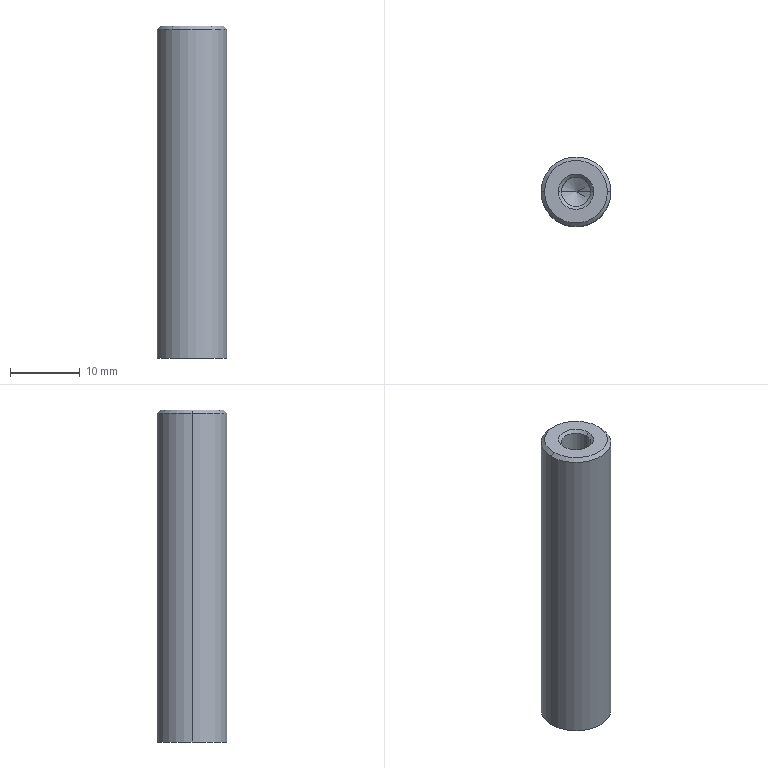Part | 1 solid | 12 faces | box 10 x 10 x 47.5 mm | volume 3479 mm3 | cone 6 | cylinder 4 | plane 2 | commonest cylinder face diameters 4.2 x2 10 x2
STEP:
#1=CARTESIAN_POINT('',(-2.1,0.,47.075));
#2=VERTEX_POINT('',#1);
#3=CARTESIAN_POINT('',(2.1,0.,47.075));
#4=VERTEX_POINT('',#3);
#5=CARTESIAN_POINT('',(0.,0.,47.075));
#6=DIRECTION('',(0.,0.,1.));
#7=DIRECTION('',(1.,0.,0.));
#8=AXIS2_PLACEMENT_3D('',#5,#6,#7);
#9=CIRCLE('',#8,2.1);
#10=EDGE_CURVE('',#2,#4,#9,.T.);
#11=ORIENTED_EDGE('',*,*,#10,.F.);
#12=CARTESIAN_POINT('',(-2.525,0.,47.5));
#13=VERTEX_POINT('',#12);
#14=CARTESIAN_POINT('',(-2.525,0.,47.5));
#15=DIRECTION('',(-0.7071,0.,0.7071));
#16=VECTOR('',#15,1000.);
#17=LINE('',#14,#16);
#18=EDGE_CURVE('',#2,#13,#17,.T.);
#19=ORIENTED_EDGE('',*,*,#18,.T.);
#20=CARTESIAN_POINT('',(2.525,0.,47.5));
#21=VERTEX_POINT('',#20);
#22=CARTESIAN_POINT('',(0.,0.,47.5));
#23=DIRECTION('',(0.,0.,1.));
#24=DIRECTION('',(1.,0.,0.));
#25=AXIS2_PLACEMENT_3D('',#22,#23,#24);
#26=CIRCLE('',#25,2.525);
#27=EDGE_CURVE('',#13,#21,#26,.T.);
#28=ORIENTED_EDGE('',*,*,#27,.T.);
#29=CARTESIAN_POINT('',(2.525,0.,47.5));
#30=DIRECTION('',(0.7071,0.,0.7071));
#31=VECTOR('',#30,1000.);
#32=LINE('',#29,#31);
#33=EDGE_CURVE('',#4,#21,#32,.T.);
#34=ORIENTED_EDGE('',*,*,#33,.F.);
#35=EDGE_LOOP('',(#11,#19,#28,#34));
#36=FACE_OUTER_BOUND('',#35,.T.);
#37=CARTESIAN_POINT('',(0.,0.,47.5));
#38=DIRECTION('',(0.,0.,1.));
#39=DIRECTION('',(1.,0.,0.));
#40=AXIS2_PLACEMENT_3D('',#37,#38,#39);
#41=CONICAL_SURFACE('',#40,2.525,0.7854);
#42=ADVANCED_FACE('',(#36),#41,.F.);
#43=CARTESIAN_POINT('',(-2.1,0.,30.1));
#44=VERTEX_POINT('',#43);
#45=CARTESIAN_POINT('',(2.1,0.,30.1));
#46=VERTEX_POINT('',#45);
#47=CARTESIAN_POINT('',(0.,0.,30.1));
#48=DIRECTION('',(0.,0.,1.));
#49=DIRECTION('',(1.,0.,0.));
#50=AXIS2_PLACEMENT_3D('',#47,#48,#49);
#51=CIRCLE('',#50,2.1);
#52=EDGE_CURVE('',#44,#46,#51,.T.);
#53=ORIENTED_EDGE('',*,*,#52,.F.);
#54=CARTESIAN_POINT('',(-2.1,0.,47.5));
#55=DIRECTION('',(0.,0.,1.));
#56=VECTOR('',#55,1000.);
#57=LINE('',#54,#56);
#58=EDGE_CURVE('',#44,#2,#57,.T.);
#59=ORIENTED_EDGE('',*,*,#58,.T.);
#60=ORIENTED_EDGE('',*,*,#10,.T.);
#61=CARTESIAN_POINT('',(2.1,0.,47.5));
#62=DIRECTION('',(0.,0.,1.));
#63=VECTOR('',#62,1000.);
#64=LINE('',#61,#63);
#65=EDGE_CURVE('',#46,#4,#64,.T.);
#66=ORIENTED_EDGE('',*,*,#65,.F.);
#67=EDGE_LOOP('',(#53,#59,#60,#66));
#68=FACE_OUTER_BOUND('',#67,.T.);
#69=CARTESIAN_POINT('',(0.,0.,47.5));
#70=DIRECTION('',(0.,0.,1.));
#71=DIRECTION('',(1.,0.,0.));
#72=AXIS2_PLACEMENT_3D('',#69,#70,#71);
#73=CYLINDRICAL_SURFACE('',#72,2.1);
#74=ADVANCED_FACE('',(#68),#73,.F.);
#75=CARTESIAN_POINT('',(0.,0.,28.838));
#76=VERTEX_POINT('',#75);
#77=CARTESIAN_POINT('',(2.1,0.,30.1));
#78=DIRECTION('',(0.8572,0.,0.515));
#79=VECTOR('',#78,1000.);
#80=LINE('',#77,#79);
#81=EDGE_CURVE('',#76,#46,#80,.T.);
#82=ORIENTED_EDGE('',*,*,#81,.F.);
#83=CARTESIAN_POINT('',(-2.1,0.,30.1));
#84=DIRECTION('',(-0.8572,0.,0.515));
#85=VECTOR('',#84,1000.);
#86=LINE('',#83,#85);
#87=EDGE_CURVE('',#76,#44,#86,.T.);
#88=ORIENTED_EDGE('',*,*,#87,.T.);
#89=ORIENTED_EDGE('',*,*,#52,.T.);
#90=EDGE_LOOP('',(#82,#88,#89));
#91=FACE_OUTER_BOUND('',#90,.T.);
#92=CARTESIAN_POINT('',(0.,0.,30.1));
#93=DIRECTION('',(0.,0.,1.));
#94=DIRECTION('',(1.,0.,0.));
#95=AXIS2_PLACEMENT_3D('',#92,#93,#94);
#96=CONICAL_SURFACE('',#95,2.1,1.03);
#97=ADVANCED_FACE('',(#91),#96,.F.);
#98=CARTESIAN_POINT('',(4.5,0.,47.5));
#99=VERTEX_POINT('',#98);
#100=CARTESIAN_POINT('',(-4.5,0.,47.5));
#101=VERTEX_POINT('',#100);
#102=CARTESIAN_POINT('',(0.,0.,47.5));
#103=DIRECTION('',(0.,0.,1.));
#104=DIRECTION('',(1.,0.,0.));
#105=AXIS2_PLACEMENT_3D('',#102,#103,#104);
#106=CIRCLE('',#105,4.5);
#107=EDGE_CURVE('',#99,#101,#106,.T.);
#108=ORIENTED_EDGE('',*,*,#107,.F.);
#109=CARTESIAN_POINT('',(5.,0.,47.));
#110=VERTEX_POINT('',#109);
#111=CARTESIAN_POINT('',(4.5,0.,47.5));
#112=DIRECTION('',(0.7071,0.,-0.7071));
#113=VECTOR('',#112,1000.);
#114=LINE('',#111,#113);
#115=EDGE_CURVE('',#99,#110,#114,.T.);
#116=ORIENTED_EDGE('',*,*,#115,.T.);
#117=CARTESIAN_POINT('',(-5.,0.,47.));
#118=VERTEX_POINT('',#117);
#119=CARTESIAN_POINT('',(0.,0.,47.));
#120=DIRECTION('',(0.,0.,-1.));
#121=DIRECTION('',(1.,0.,0.));
#122=AXIS2_PLACEMENT_3D('',#119,#120,#121);
#123=CIRCLE('',#122,5.);
#124=EDGE_CURVE('',#118,#110,#123,.T.);
#125=ORIENTED_EDGE('',*,*,#124,.F.);
#126=CARTESIAN_POINT('',(-4.5,0.,47.5));
#127=DIRECTION('',(-0.7071,0.,-0.7071));
#128=VECTOR('',#127,1000.);
#129=LINE('',#126,#128);
#130=EDGE_CURVE('',#101,#118,#129,.T.);
#131=ORIENTED_EDGE('',*,*,#130,.F.);
#132=EDGE_LOOP('',(#108,#116,#125,#131));
#133=FACE_OUTER_BOUND('',#132,.T.);
#134=CARTESIAN_POINT('',(0.,0.,47.5));
#135=DIRECTION('',(0.,0.,-1.));
#136=DIRECTION('',(-1.,0.,0.));
#137=AXIS2_PLACEMENT_3D('',#134,#135,#136);
#138=CONICAL_SURFACE('',#137,4.5,0.7854);
#139=ADVANCED_FACE('',(#133),#138,.T.);
#140=ORIENTED_EDGE('',*,*,#124,.T.);
#141=CARTESIAN_POINT('',(5.,0.,0.));
#142=VERTEX_POINT('',#141);
#143=CARTESIAN_POINT('',(5.,0.,47.5));
#144=DIRECTION('',(0.,0.,-1.));
#145=VECTOR('',#144,1000.);
#146=LINE('',#143,#145);
#147=EDGE_CURVE('',#110,#142,#146,.T.);
#148=ORIENTED_EDGE('',*,*,#147,.T.);
#149=CARTESIAN_POINT('',(-5.,0.,0.));
#150=VERTEX_POINT('',#149);
#151=CARTESIAN_POINT('',(0.,0.,0.));
#152=DIRECTION('',(0.,0.,1.));
#153=DIRECTION('',(1.,0.,0.));
#154=AXIS2_PLACEMENT_3D('',#151,#152,#153);
#155=CIRCLE('',#154,5.);
#156=EDGE_CURVE('',#142,#150,#155,.T.);
#157=ORIENTED_EDGE('',*,*,#156,.T.);
#158=CARTESIAN_POINT('',(-5.,0.,47.5));
#159=DIRECTION('',(0.,0.,-1.));
#160=VECTOR('',#159,1000.);
#161=LINE('',#158,#160);
#162=EDGE_CURVE('',#118,#150,#161,.T.);
#163=ORIENTED_EDGE('',*,*,#162,.F.);
#164=EDGE_LOOP('',(#140,#148,#157,#163));
#165=FACE_OUTER_BOUND('',#164,.T.);
#166=CARTESIAN_POINT('',(0.,0.,47.5));
#167=DIRECTION('',(0.,0.,-1.));
#168=DIRECTION('',(-1.,0.,0.));
#169=AXIS2_PLACEMENT_3D('',#166,#167,#168);
#170=CYLINDRICAL_SURFACE('',#169,5.);
#171=ADVANCED_FACE('',(#165),#170,.T.);
#172=ORIENTED_EDGE('',*,*,#147,.F.);
#173=CARTESIAN_POINT('',(0.,0.,47.));
#174=DIRECTION('',(0.,0.,-1.));
#175=DIRECTION('',(1.,0.,0.));
#176=AXIS2_PLACEMENT_3D('',#173,#174,#175);
#177=CIRCLE('',#176,5.);
#178=EDGE_CURVE('',#110,#118,#177,.T.);
#179=ORIENTED_EDGE('',*,*,#178,.T.);
#180=ORIENTED_EDGE('',*,*,#162,.T.);
#181=CARTESIAN_POINT('',(0.,0.,0.));
#182=DIRECTION('',(0.,0.,1.));
#183=DIRECTION('',(1.,0.,0.));
#184=AXIS2_PLACEMENT_3D('',#181,#182,#183);
#185=CIRCLE('',#184,5.);
#186=EDGE_CURVE('',#150,#142,#185,.T.);
#187=ORIENTED_EDGE('',*,*,#186,.T.);
#188=EDGE_LOOP('',(#172,#179,#180,#187));
#189=FACE_OUTER_BOUND('',#188,.T.);
#190=CARTESIAN_POINT('',(0.,0.,47.5));
#191=DIRECTION('',(0.,0.,-1.));
#192=DIRECTION('',(-1.,0.,0.));
#193=AXIS2_PLACEMENT_3D('',#190,#191,#192);
#194=CYLINDRICAL_SURFACE('',#193,5.);
#195=ADVANCED_FACE('',(#189),#194,.T.);
#196=CARTESIAN_POINT('',(0.,0.,47.5));
#197=DIRECTION('',(0.,0.,1.));
#198=DIRECTION('',(1.,0.,0.));
#199=AXIS2_PLACEMENT_3D('',#196,#197,#198);
#200=CIRCLE('',#199,4.5);
#201=EDGE_CURVE('',#101,#99,#200,.T.);
#202=ORIENTED_EDGE('',*,*,#201,.T.);
#203=ORIENTED_EDGE('',*,*,#107,.T.);
#204=EDGE_LOOP('',(#202,#203));
#205=FACE_OUTER_BOUND('',#204,.T.);
#206=CARTESIAN_POINT('',(0.,0.,47.5));
#207=DIRECTION('',(0.,0.,1.));
#208=DIRECTION('',(1.,0.,0.));
#209=AXIS2_PLACEMENT_3D('',#206,#207,#208);
#210=CIRCLE('',#209,2.525);
#211=EDGE_CURVE('',#21,#13,#210,.T.);
#212=ORIENTED_EDGE('',*,*,#211,.F.);
#213=ORIENTED_EDGE('',*,*,#27,.F.);
#214=EDGE_LOOP('',(#212,#213));
#215=FACE_BOUND('',#214,.T.);
#216=CARTESIAN_POINT('',(0.,0.,47.5));
#217=DIRECTION('',(0.,0.,1.));
#218=DIRECTION('',(1.,0.,0.));
#219=AXIS2_PLACEMENT_3D('',#216,#217,#218);
#220=PLANE('',#219);
#221=ADVANCED_FACE('',(#205,#215),#220,.T.);
#222=ORIENTED_EDGE('',*,*,#186,.F.);
#223=ORIENTED_EDGE('',*,*,#156,.F.);
#224=EDGE_LOOP('',(#222,#223));
#225=FACE_OUTER_BOUND('',#224,.T.);
#226=CARTESIAN_POINT('',(0.,0.,0.));
#227=DIRECTION('',(0.,0.,1.));
#228=DIRECTION('',(1.,0.,0.));
#229=AXIS2_PLACEMENT_3D('',#226,#227,#228);
#230=PLANE('',#229);
#231=ADVANCED_FACE('',(#225),#230,.F.);
#232=ORIENTED_EDGE('',*,*,#115,.F.);
#233=ORIENTED_EDGE('',*,*,#201,.F.);
#234=ORIENTED_EDGE('',*,*,#130,.T.);
#235=ORIENTED_EDGE('',*,*,#178,.F.);
#236=EDGE_LOOP('',(#232,#233,#234,#235));
#237=FACE_OUTER_BOUND('',#236,.T.);
#238=CARTESIAN_POINT('',(0.,0.,47.5));
#239=DIRECTION('',(0.,0.,-1.));
#240=DIRECTION('',(-1.,0.,0.));
#241=AXIS2_PLACEMENT_3D('',#238,#239,#240);
#242=CONICAL_SURFACE('',#241,4.5,0.7854);
#243=ADVANCED_FACE('',(#237),#242,.T.);
#244=ORIENTED_EDGE('',*,*,#87,.F.);
#245=ORIENTED_EDGE('',*,*,#81,.T.);
#246=CARTESIAN_POINT('',(0.,0.,30.1));
#247=DIRECTION('',(0.,0.,1.));
#248=DIRECTION('',(1.,0.,0.));
#249=AXIS2_PLACEMENT_3D('',#246,#247,#248);
#250=CIRCLE('',#249,2.1);
#251=EDGE_CURVE('',#46,#44,#250,.T.);
#252=ORIENTED_EDGE('',*,*,#251,.T.);
#253=EDGE_LOOP('',(#244,#245,#252));
#254=FACE_OUTER_BOUND('',#253,.T.);
#255=CARTESIAN_POINT('',(0.,0.,30.1));
#256=DIRECTION('',(0.,0.,1.));
#257=DIRECTION('',(1.,0.,0.));
#258=AXIS2_PLACEMENT_3D('',#255,#256,#257);
#259=CONICAL_SURFACE('',#258,2.1,1.03);
#260=ADVANCED_FACE('',(#254),#259,.F.);
#261=ORIENTED_EDGE('',*,*,#58,.F.);
#262=ORIENTED_EDGE('',*,*,#251,.F.);
#263=ORIENTED_EDGE('',*,*,#65,.T.);
#264=CARTESIAN_POINT('',(0.,0.,47.075));
#265=DIRECTION('',(0.,0.,1.));
#266=DIRECTION('',(1.,0.,0.));
#267=AXIS2_PLACEMENT_3D('',#264,#265,#266);
#268=CIRCLE('',#267,2.1);
#269=EDGE_CURVE('',#4,#2,#268,.T.);
#270=ORIENTED_EDGE('',*,*,#269,.T.);
#271=EDGE_LOOP('',(#261,#262,#263,#270));
#272=FACE_OUTER_BOUND('',#271,.T.);
#273=CARTESIAN_POINT('',(0.,0.,47.5));
#274=DIRECTION('',(0.,0.,1.));
#275=DIRECTION('',(1.,0.,0.));
#276=AXIS2_PLACEMENT_3D('',#273,#274,#275);
#277=CYLINDRICAL_SURFACE('',#276,2.1);
#278=ADVANCED_FACE('',(#272),#277,.F.);
#279=ORIENTED_EDGE('',*,*,#18,.F.);
#280=ORIENTED_EDGE('',*,*,#269,.F.);
#281=ORIENTED_EDGE('',*,*,#33,.T.);
#282=ORIENTED_EDGE('',*,*,#211,.T.);
#283=EDGE_LOOP('',(#279,#280,#281,#282));
#284=FACE_OUTER_BOUND('',#283,.T.);
#285=CARTESIAN_POINT('',(0.,0.,47.5));
#286=DIRECTION('',(0.,0.,1.));
#287=DIRECTION('',(1.,0.,0.));
#288=AXIS2_PLACEMENT_3D('',#285,#286,#287);
#289=CONICAL_SURFACE('',#288,2.525,0.7854);
#290=ADVANCED_FACE('',(#284),#289,.F.);
#291=CLOSED_SHELL('',(#42,#74,#97,#139,#171,#195,#221,#231,#243,#260,#278,#290));
#292=MANIFOLD_SOLID_BREP('',#291);
#293=CARTESIAN_POINT('',(0.,0.,0.));
#294=DIRECTION('',(0.,0.,1.));
#295=DIRECTION('',(1.,0.,0.));
#296=AXIS2_PLACEMENT_3D('',#293,#294,#295);
#297=(LENGTH_UNIT()NAMED_UNIT(*)SI_UNIT(.MILLI.,.METRE.));
#298=UNCERTAINTY_MEASURE_WITH_UNIT(LENGTH_MEASURE(0.00001),#297,'','');
#299=(NAMED_UNIT(*)PLANE_ANGLE_UNIT()SI_UNIT($,.RADIAN.));
#300=(NAMED_UNIT(*)SI_UNIT($,.STERADIAN.)SOLID_ANGLE_UNIT());
#301=(GEOMETRIC_REPRESENTATION_CONTEXT(3)GLOBAL_UNCERTAINTY_ASSIGNED_CONTEXT((#298))GLOBAL_UNIT_ASSIGNED_CONTEXT((#297,#299,#300))REPRESENTATION_CONTEXT('',''));
#302=ADVANCED_BREP_SHAPE_REPRESENTATION('',(#292,#296),#301);